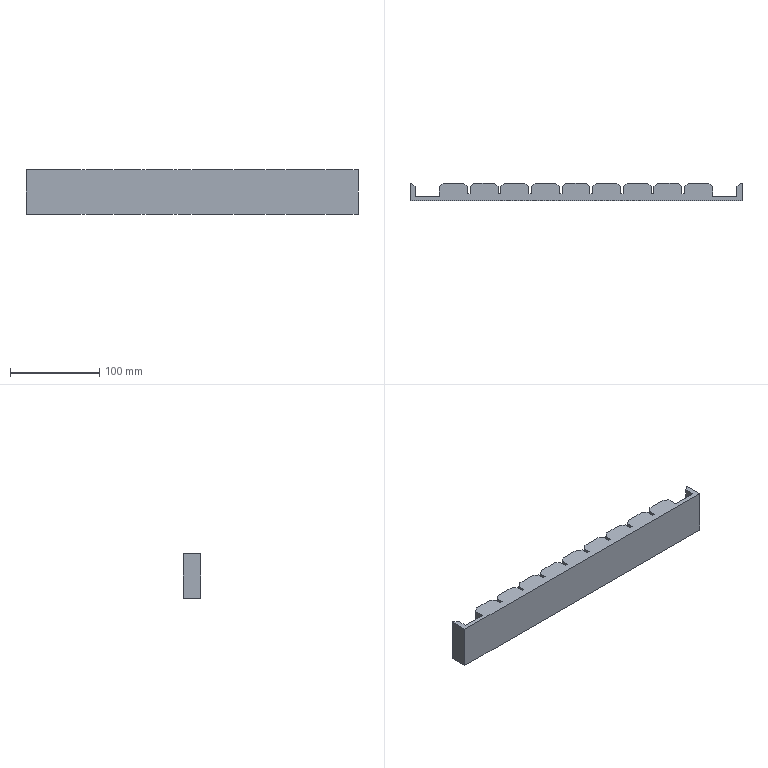NC program | NX | posted with a generic post | part box 372.9 x 20 x 50 mm
Lines 1 to 1463 of 3956:
N10 G17 G21 G94 G90
(FLOOR_WALL , TOOL : D6)
N12 T12 M6
N14 G54
N16 G17 G0 G90 X-164.156 Y-29.5 S9500 M3
N18 G43 Z30. H12
N20 Z0.904
N22 G94 G1 Z-0.596 F2500.
N24 X-166.58 Y-25.3
N26 G3 X-167.1 Y-25. R0.6
N28 G1 X-177.6
N30 Y25.
N32 X-156.6
N34 Y-25.
N36 X-167.1
N38 Y-22.
N40 X-174.6
N42 Y22.
N44 X-159.6
N46 Y-22.
N48 X-167.1
N50 Y-19.
N52 X-171.6
N54 Y19.
N56 X-162.6
N58 Y-19.
N60 X-167.1
N62 Y-16.
N64 X-168.6
N66 Y16.
N68 X-165.6
N70 Y-16.
N72 X-167.1
N74 G3 X-167.62 Y-16.3 R0.6
N76 G1 Z0.904
N78 G0 X-164.156 Y-29.5 Z0.308
N80 G1 Z-1.192
N82 X-166.58 Y-25.3
N84 G3 X-167.1 Y-25. R0.6
N86 G1 X-177.6
N88 Y25.
N90 X-156.6
N92 Y-25.
N94 X-167.1
N96 Y-22.
N98 X-174.6
N100 Y22.
N102 X-159.6
N104 Y-22.
N106 X-167.1
N108 Y-19.
N110 X-171.6
N112 Y19.
N114 X-162.6
N116 Y-19.
N118 X-167.1
N120 Y-16.
N122 X-168.6
N124 Y16.
N126 X-165.6
N128 Y-16.
N130 X-167.1
N132 G3 X-167.62 Y-16.3 R0.6
N134 G1 Z0.308
N136 G0 X-164.156 Y-29.5 Z-0.288
N138 G1 Z-1.788
N140 X-166.58 Y-25.3
N142 G3 X-167.1 Y-25. R0.6
N144 G1 X-177.6
N146 Y25.
N148 X-156.6
N150 Y-25.
N152 X-167.1
N154 Y-22.
N156 X-174.6
N158 Y22.
N160 X-159.6
N162 Y-22.
N164 X-167.1
N166 Y-19.
N168 X-171.6
N170 Y19.
N172 X-162.6
N174 Y-19.
N176 X-167.1
N178 Y-16.
N180 X-168.6
N182 Y16.
N184 X-165.6
N186 Y-16.
N188 X-167.1
N190 G3 X-167.62 Y-16.3 R0.6
N192 G1 Z-0.288
N194 G0 X-164.156 Y-29.5 Z-0.884
N196 G1 Z-2.384
N198 X-166.58 Y-25.3
N200 G3 X-167.1 Y-25. R0.6
N202 G1 X-177.6
N204 Y25.
N206 X-156.6
N208 Y-25.
N210 X-167.1
N212 Y-22.
N214 X-174.6
N216 Y22.
N218 X-159.6
N220 Y-22.
N222 X-167.1
N224 Y-19.
N226 X-171.6
N228 Y19.
N230 X-162.6
N232 Y-19.
N234 X-167.1
N236 Y-16.
N238 X-168.6
N240 Y16.
N242 X-165.6
N244 Y-16.
N246 X-167.1
N248 G3 X-167.62 Y-16.3 R0.6
N250 G1 Z-0.884
N252 G0 X-164.156 Y-29.5 Z-1.48
N254 G1 Z-2.98
N256 X-166.58 Y-25.3
N258 G3 X-167.1 Y-25. R0.6
N260 G1 X-177.6
N262 Y25.
N264 X-156.6
N266 Y-25.
N268 X-167.1
N270 Y-22.
N272 X-174.6
N274 Y22.
N276 X-159.6
N278 Y-22.
N280 X-167.1
N282 Y-19.
N284 X-171.6
N286 Y19.
N288 X-162.6
N290 Y-19.
N292 X-167.1
N294 Y-16.
N296 X-168.6
N298 Y16.
N300 X-165.6
N302 Y-16.
N304 X-167.1
N306 G3 X-167.62 Y-16.3 R0.6
N308 G1 Z-1.48
N310 G0 X-164.156 Y-29.5 Z-2.076
N312 G1 Z-3.576
N314 X-166.58 Y-25.3
N316 G3 X-167.1 Y-25. R0.6
N318 G1 X-177.6
N320 Y25.
N322 X-156.6
N324 Y-25.
N326 X-167.1
N328 Y-22.
N330 X-174.6
N332 Y22.
N334 X-159.6
N336 Y-22.
N338 X-167.1
N340 Y-19.
N342 X-171.6
N344 Y19.
N346 X-162.6
N348 Y-19.
N350 X-167.1
N352 Y-16.
N354 X-168.6
N356 Y16.
N358 X-165.6
N360 Y-16.
N362 X-167.1
N364 G3 X-167.62 Y-16.3 R0.6
N366 G1 Z-2.076
N368 G0 X-164.156 Y-29.5 Z-2.672
N370 G1 Z-4.172
N372 X-166.58 Y-25.3
N374 G3 X-167.1 Y-25. R0.6
N376 G1 X-177.6
N378 Y25.
N380 X-156.6
N382 Y-25.
N384 X-167.1
N386 Y-22.
N388 X-174.6
N390 Y22.
N392 X-159.6
N394 Y-22.
N396 X-167.1
N398 Y-19.
N400 X-171.6
N402 Y19.
N404 X-162.6
N406 Y-19.
N408 X-167.1
N410 Y-16.
N412 X-168.6
N414 Y16.
N416 X-165.6
N418 Y-16.
N420 X-167.1
N422 G3 X-167.62 Y-16.3 R0.6
N424 G1 Z-2.672
N426 G0 X-164.156 Y-29.5 Z-3.268
N428 G1 Z-4.768
N430 X-166.58 Y-25.3
N432 G3 X-167.1 Y-25. R0.6
N434 G1 X-177.6
N436 Y25.
N438 X-156.6
N440 Y-25.
N442 X-167.1
N444 Y-22.
N446 X-174.6
N448 Y22.
N450 X-159.6
N452 Y-22.
N454 X-167.1
N456 Y-19.
N458 X-171.6
N460 Y19.
N462 X-162.6
N464 Y-19.
N466 X-167.1
N468 Y-16.
N470 X-168.6
N472 Y16.
N474 X-165.6
N476 Y-16.
N478 X-167.1
N480 G3 X-167.62 Y-16.3 R0.6
N482 G1 Z-3.268
N484 G0 X-164.156 Y-29.5 Z-3.864
N486 G1 Z-5.364
N488 X-166.58 Y-25.3
N490 G3 X-167.1 Y-25. R0.6
N492 G1 X-177.6
N494 Y25.
N496 X-156.6
N498 Y-25.
N500 X-167.1
N502 Y-22.
N504 X-174.6
N506 Y22.
N508 X-159.6
N510 Y-22.
N512 X-167.1
N514 Y-19.
N516 X-171.6
N518 Y19.
N520 X-162.6
N522 Y-19.
N524 X-167.1
N526 Y-16.
N528 X-168.6
N530 Y16.
N532 X-165.6
N534 Y-16.
N536 X-167.1
N538 G3 X-167.62 Y-16.3 R0.6
N540 G1 Z-3.864
N542 G0 X-164.156 Y-29.5 Z-4.46
N544 G1 Z-5.96
N546 X-166.58 Y-25.3
N548 G3 X-167.1 Y-25. R0.6
N550 G1 X-177.6
N552 Y25.
N554 X-156.6
N556 Y-25.
N558 X-167.1
N560 Y-22.
N562 X-174.6
N564 Y22.
N566 X-159.6
N568 Y-22.
N570 X-167.1
N572 Y-19.
N574 X-171.6
N576 Y19.
N578 X-162.6
N580 Y-19.
N582 X-167.1
N584 Y-16.
N586 X-168.6
N588 Y16.
N590 X-165.6
N592 Y-16.
N594 X-167.1
N596 G3 X-167.62 Y-16.3 R0.6
N598 G1 Z-4.46
N600 G0 X-164.156 Y-29.5 Z-5.056
N602 G1 Z-6.556
N604 X-166.58 Y-25.3
N606 G3 X-167.1 Y-25. R0.6
N608 G1 X-177.6
N610 Y25.
N612 X-156.6
N614 Y-25.
N616 X-167.1
N618 Y-22.
N620 X-174.6
N622 Y22.
N624 X-159.6
N626 Y-22.
N628 X-167.1
N630 Y-19.
N632 X-171.6
N634 Y19.
N636 X-162.6
N638 Y-19.
N640 X-167.1
N642 Y-16.
N644 X-168.6
N646 Y16.
N648 X-165.6
N650 Y-16.
N652 X-167.1
N654 G3 X-167.62 Y-16.3 R0.6
N656 G1 Z-5.056
N658 G0 X-164.156 Y-29.5 Z-5.652
N660 G1 Z-7.152
N662 X-166.58 Y-25.3
N664 G3 X-167.1 Y-25. R0.6
N666 G1 X-177.6
N668 Y25.
N670 X-156.6
N672 Y-25.
N674 X-167.1
N676 Y-22.
N678 X-174.6
N680 Y22.
N682 X-159.6
N684 Y-22.
N686 X-167.1
N688 Y-19.
N690 X-171.6
N692 Y19.
N694 X-162.6
N696 Y-19.
N698 X-167.1
N700 Y-16.
N702 X-168.6
N704 Y16.
N706 X-165.6
N708 Y-16.
N710 X-167.1
N712 G3 X-167.62 Y-16.3 R0.6
N714 G1 Z-5.652
N716 G0 X-164.156 Y-29.5 Z-6.248
N718 G1 Z-7.748
N720 X-166.58 Y-25.3
N722 G3 X-167.1 Y-25. R0.6
N724 G1 X-177.6
N726 Y25.
N728 X-156.6
N730 Y-25.
N732 X-167.1
N734 Y-22.
N736 X-174.6
N738 Y22.
N740 X-159.6
N742 Y-22.
N744 X-167.1
N746 Y-19.
N748 X-171.6
N750 Y19.
N752 X-162.6
N754 Y-19.
N756 X-167.1
N758 Y-16.
N760 X-168.6
N762 Y16.
N764 X-165.6
N766 Y-16.
N768 X-167.1
N770 G3 X-167.62 Y-16.3 R0.6
N772 G1 Z-6.248
N774 G0 X-164.156 Y-29.5 Z-6.844
N776 G1 Z-8.344
N778 X-166.58 Y-25.3
N780 G3 X-167.1 Y-25. R0.6
N782 G1 X-177.6
N784 Y25.
N786 X-156.6
N788 Y-25.
N790 X-167.1
N792 Y-22.
N794 X-174.6
N796 Y22.
N798 X-159.6
N800 Y-22.
N802 X-167.1
N804 Y-19.
N806 X-171.6
N808 Y19.
N810 X-162.6
N812 Y-19.
N814 X-167.1
N816 Y-16.
N818 X-168.6
N820 Y16.
N822 X-165.6
N824 Y-16.
N826 X-167.1
N828 G3 X-167.62 Y-16.3 R0.6
N830 G1 Z-6.844
N832 G0 X-164.156 Y-29.5 Z-7.44
N834 G1 Z-8.94
N836 X-166.58 Y-25.3
N838 G3 X-167.1 Y-25. R0.6
N840 G1 X-177.6
N842 Y25.
N844 X-156.6
N846 Y-25.
N848 X-167.1
N850 Y-22.
N852 X-174.6
N854 Y22.
N856 X-159.6
N858 Y-22.
N860 X-167.1
N862 Y-19.
N864 X-171.6
N866 Y19.
N868 X-162.6
N870 Y-19.
N872 X-167.1
N874 Y-16.
N876 X-168.6
N878 Y16.
N880 X-165.6
N882 Y-16.
N884 X-167.1
N886 G3 X-167.62 Y-16.3 R0.6
N888 G1 Z-7.44
N890 G0 X-164.156 Y-29.5 Z-8.036
N892 G1 Z-9.536
N894 X-166.58 Y-25.3
N896 G3 X-167.1 Y-25. R0.6
N898 G1 X-177.6
N900 Y25.
N902 X-156.6
N904 Y-25.
N906 X-167.1
N908 Y-22.
N910 X-174.6
N912 Y22.
N914 X-159.6
N916 Y-22.
N918 X-167.1
N920 Y-19.
N922 X-171.6
N924 Y19.
N926 X-162.6
N928 Y-19.
N930 X-167.1
N932 Y-16.
N934 X-168.6
N936 Y16.
N938 X-165.6
N940 Y-16.
N942 X-167.1
N944 G3 X-167.62 Y-16.3 R0.6
N946 G1 Z-8.036
N948 G0 X-164.156 Y-29.5 Z-8.632
N950 G1 Z-10.132
N952 X-166.58 Y-25.3
N954 G3 X-167.1 Y-25. R0.6
N956 G1 X-177.6
N958 Y25.
N960 X-156.6
N962 Y-25.
N964 X-167.1
N966 Y-22.
N968 X-174.6
N970 Y22.
N972 X-159.6
N974 Y-22.
N976 X-167.1
N978 Y-19.
N980 X-171.6
N982 Y19.
N984 X-162.6
N986 Y-19.
N988 X-167.1
N990 Y-16.
N992 X-168.6
N994 Y16.
N996 X-165.6
N998 Y-16.
N1000 X-167.1
N1002 G3 X-167.62 Y-16.3 R0.6
N1004 G1 Z-8.632
N1006 G0 X-164.156 Y-29.5 Z-9.228
N1008 G1 Z-10.728
N1010 X-166.58 Y-25.3
N1012 G3 X-167.1 Y-25. R0.6
N1014 G1 X-177.6
N1016 Y25.
N1018 X-156.6
N1020 Y-25.
N1022 X-167.1
N1024 Y-22.
N1026 X-174.6
N1028 Y22.
N1030 X-159.6
N1032 Y-22.
N1034 X-167.1
N1036 Y-19.
N1038 X-171.6
N1040 Y19.
N1042 X-162.6
N1044 Y-19.
N1046 X-167.1
N1048 Y-16.
N1050 X-168.6
N1052 Y16.
N1054 X-165.6
N1056 Y-16.
N1058 X-167.1
N1060 G3 X-167.62 Y-16.3 R0.6
N1062 G1 Z-9.228
N1064 G0 X-164.156 Y-29.5 Z-9.824
N1066 G1 Z-11.324
N1068 X-166.58 Y-25.3
N1070 G3 X-167.1 Y-25. R0.6
N1072 G1 X-177.6
N1074 Y25.
N1076 X-156.6
N1078 Y-25.
N1080 X-167.1
N1082 Y-22.
N1084 X-174.6
N1086 Y22.
N1088 X-159.6
N1090 Y-22.
N1092 X-167.1
N1094 Y-19.
N1096 X-171.6
N1098 Y19.
N1100 X-162.6
N1102 Y-19.
N1104 X-167.1
N1106 Y-16.
N1108 X-168.6
N1110 Y16.
N1112 X-165.6
N1114 Y-16.
N1116 X-167.1
N1118 G3 X-167.62 Y-16.3 R0.6
N1120 G1 Z-9.824
N1122 G0 X-164.156 Y-29.5 Z-10.42
N1124 G1 Z-11.92
N1126 X-166.58 Y-25.3
N1128 G3 X-167.1 Y-25. R0.6
N1130 G1 X-177.6
N1132 Y25.
N1134 X-156.6
N1136 Y-25.
N1138 X-167.1
N1140 Y-22.
N1142 X-174.6
N1144 Y22.
N1146 X-159.6
N1148 Y-22.
N1150 X-167.1
N1152 Y-19.
N1154 X-171.6
N1156 Y19.
N1158 X-162.6
N1160 Y-19.
N1162 X-167.1
N1164 Y-16.
N1166 X-168.6
N1168 Y16.
N1170 X-165.6
N1172 Y-16.
N1174 X-167.1
N1176 G3 X-167.62 Y-16.3 R0.6
N1178 G1 Z-10.42
N1180 G0 X-164.156 Y-29.5 Z-11.016
N1182 G1 Z-12.516
N1184 X-166.58 Y-25.3
N1186 G3 X-167.1 Y-25. R0.6
N1188 G1 X-177.6
N1190 Y25.
N1192 X-156.6
N1194 Y-25.
N1196 X-167.1
N1198 Y-22.
N1200 X-174.6
N1202 Y22.
N1204 X-159.6
N1206 Y-22.
N1208 X-167.1
N1210 Y-19.
N1212 X-171.6
N1214 Y19.
N1216 X-162.6
N1218 Y-19.
N1220 X-167.1
N1222 Y-16.
N1224 X-168.6
N1226 Y16.
N1228 X-165.6
N1230 Y-16.
N1232 X-167.1
N1234 G3 X-167.62 Y-16.3 R0.6
N1236 G1 Z-11.016
N1238 G0 X-164.156 Y-29.5 Z-11.612
N1240 G1 Z-13.112
N1242 X-166.58 Y-25.3
N1244 G3 X-167.1 Y-25. R0.6
N1246 G1 X-177.6
N1248 Y25.
N1250 X-156.6
N1252 Y-25.
N1254 X-167.1
N1256 Y-22.
N1258 X-174.6
N1260 Y22.
N1262 X-159.6
N1264 Y-22.
N1266 X-167.1
N1268 Y-19.
N1270 X-171.6
N1272 Y19.
N1274 X-162.6
N1276 Y-19.
N1278 X-167.1
N1280 Y-16.
N1282 X-168.6
N1284 Y16.
N1286 X-165.6
N1288 Y-16.
N1290 X-167.1
N1292 G3 X-167.62 Y-16.3 R0.6
N1294 G1 Z-11.612
N1296 G0 X-164.156 Y-29.5 Z-12.208
N1298 G1 Z-13.708
N1300 X-166.58 Y-25.3
N1302 G3 X-167.1 Y-25. R0.6
N1304 G1 X-177.6
N1306 Y25.
N1308 X-156.6
N1310 Y-25.
N1312 X-167.1
N1314 Y-22.
N1316 X-174.6
N1318 Y22.
N1320 X-159.6
N1322 Y-22.
N1324 X-167.1
N1326 Y-19.
N1328 X-171.6
N1330 Y19.
N1332 X-162.6
N1334 Y-19.
N1336 X-167.1
N1338 Y-16.
N1340 X-168.6
N1342 Y16.
N1344 X-165.6
N1346 Y-16.
N1348 X-167.1
N1350 G3 X-167.62 Y-16.3 R0.6
N1352 G1 Z-12.208
N1354 G0 X-164.156 Y-29.5 Z-12.804
N1356 G1 Z-14.304
N1358 X-166.58 Y-25.3
N1360 G3 X-167.1 Y-25. R0.6
N1362 G1 X-177.6
N1364 Y25.
N1366 X-156.6
N1368 Y-25.
N1370 X-167.1
N1372 Y-22.
N1374 X-174.6
N1376 Y22.
N1378 X-159.6
N1380 Y-22.
N1382 X-167.1
N1384 Y-19.
N1386 X-171.6
N1388 Y19.
N1390 X-162.6
N1392 Y-19.
N1394 X-167.1
N1396 Y-16.
N1398 X-168.6
N1400 Y16.
N1402 X-165.6
N1404 Y-16.
N1406 X-167.1
N1408 G3 X-167.62 Y-16.3 R0.6
N1410 G1 Z-12.804
N1412 G0 X-164.156 Y-29.5 Z-13.4
N1414 G1 Z-14.9
N1416 X-166.58 Y-25.3
N1418 G3 X-167.1 Y-25. R0.6
N1420 G1 X-177.6
N1422 Y25.
N1424 X-156.6
N1426 Y-25.
N1428 X-167.1
N1430 Y-22.
N1432 X-174.6
N1434 Y22.
N1436 X-159.6
N1438 Y-22.
N1440 X-167.1
N1442 Y-19.
N1444 X-171.6
N1446 Y19.
N1448 X-162.6
N1450 Y-19.
N1452 X-167.1
N1454 Y-16.
N1456 X-168.6
N1458 Y16.
N1460 X-165.6
N1462 Y-16.
N1464 X-167.1
N1466 G3 X-167.62 Y-16.3 R0.6
N1468 G1 Z-13.4
N1470 G0 Z30.
N1472 X170.044 Y-29.5
N1474 Z0.904
N1476 G1 Z-0.596
N1478 X167.62 Y-25.3
N1480 G3 X167.1 Y-25. R0.6
N1482 G1 X156.6
N1484 Y25.
N1486 X177.6
N1488 Y-25.
N1490 X167.1
N1492 Y-22.
N1494 X159.6
N1496 Y22.
N1498 X174.6
N1500 Y-22.
N1502 X167.1
N1504 Y-19.
N1506 X162.6
N1508 Y19.
N1510 X171.6
N1512 Y-19.
N1514 X167.1
N1516 Y-16.
N1518 X165.6
N1520 Y16.
N1522 X168.6
N1524 Y-16.
N1526 X167.1
N1528 G3 X166.58 Y-16.3 R0.6
N1530 G1 Z0.904
N1532 G0 X170.044 Y-29.5 Z0.308
N1534 G1 Z-1.192
N1536 X167.62 Y-25.3
N1538 G3 X167.1 Y-25. R0.6
N1540 G1 X156.6
N1542 Y25.
N1544 X177.6
N1546 Y-25.
N1548 X167.1
N1550 Y-22.
N1552 X159.6
N1554 Y22.
N1556 X174.6
N1558 Y-22.
N1560 X167.1
N1562 Y-19.
N1564 X162.6
N1566 Y19.
N1568 X171.6
N1570 Y-19.
N1572 X167.1
N1574 Y-16.
N1576 X165.6
N1578 Y16.
N1580 X168.6
N1582 Y-16.
N1584 X167.1
N1586 G3 X166.58 Y-16.3 R0.6
N1588 G1 Z0.308
N1590 G0 X170.044 Y-29.5 Z-0.288
N1592 G1 Z-1.788
N1594 X167.62 Y-25.3
N1596 G3 X167.1 Y-25. R0.6
N1598 G1 X156.6
N1600 Y25.
N1602 X177.6
N1604 Y-25.
N1606 X167.1
N1608 Y-22.
N1610 X159.6
N1612 Y22.
N1614 X174.6
N1616 Y-22.
N1618 X167.1
N1620 Y-19.
N1622 X162.6
N1624 Y19.
N1626 X171.6
N1628 Y-19.
N1630 X167.1
N1632 Y-16.
N1634 X165.6
N1636 Y16.
N1638 X168.6
N1640 Y-16.
N1642 X167.1
N1644 G3 X166.58 Y-16.3 R0.6
N1646 G1 Z-0.288
N1648 G0 X170.044 Y-29.5 Z-0.884
N1650 G1 Z-2.384
N1652 X167.62 Y-25.3
N1654 G3 X167.1 Y-25. R0.6
N1656 G1 X156.6
N1658 Y25.
N1660 X177.6
N1662 Y-25.
N1664 X167.1
N1666 Y-22.
N1668 X159.6
N1670 Y22.
N1672 X174.6
N1674 Y-22.
N1676 X167.1
N1678 Y-19.
N1680 X162.6
N1682 Y19.
N1684 X171.6
N1686 Y-19.
N1688 X167.1
N1690 Y-16.
N1692 X165.6
N1694 Y16.
N1696 X168.6
N1698 Y-16.
N1700 X167.1
N1702 G3 X166.58 Y-16.3 R0.6
N1704 G1 Z-0.884
N1706 G0 X170.044 Y-29.5 Z-1.48
N1708 G1 Z-2.98
N1710 X167.62 Y-25.3
N1712 G3 X167.1 Y-25. R0.6
N1714 G1 X156.6
N1716 Y25.
N1718 X177.6
N1720 Y-25.
N1722 X167.1
N1724 Y-22.
N1726 X159.6
N1728 Y22.
N1730 X174.6
N1732 Y-22.
N1734 X167.1
N1736 Y-19.
N1738 X162.6
N1740 Y19.
N1742 X171.6
N1744 Y-19.
N1746 X167.1
N1748 Y-16.
N1750 X165.6
N1752 Y16.
N1754 X168.6
N1756 Y-16.
N1758 X167.1
N1760 G3 X166.58 Y-16.3 R0.6
N1762 G1 Z-1.48
N1764 G0 X170.044 Y-29.5 Z-2.076
N1766 G1 Z-3.576
N1768 X167.62 Y-25.3
N1770 G3 X167.1 Y-25. R0.6
N1772 G1 X156.6
N1774 Y25.
N1776 X177.6
N1778 Y-25.
N1780 X167.1
N1782 Y-22.
N1784 X159.6
N1786 Y22.
N1788 X174.6
N1790 Y-22.
N1792 X167.1
N1794 Y-19.
N1796 X162.6
N1798 Y19.
N1800 X171.6
N1802 Y-19.
N1804 X167.1
N1806 Y-16.
N1808 X165.6
N1810 Y16.
N1812 X168.6
N1814 Y-16.
N1816 X167.1
N1818 G3 X166.58 Y-16.3 R0.6
N1820 G1 Z-2.076
N1822 G0 X170.044 Y-29.5 Z-2.672
N1824 G1 Z-4.172
N1826 X167.62 Y-25.3
N1828 G3 X167.1 Y-25. R0.6
N1830 G1 X156.6
N1832 Y25.
N1834 X177.6
N1836 Y-25.
N1838 X167.1
N1840 Y-22.
N1842 X159.6
N1844 Y22.
N1846 X174.6
N1848 Y-22.
N1850 X167.1
N1852 Y-19.
N1854 X162.6
N1856 Y19.
N1858 X171.6
N1860 Y-19.
N1862 X167.1
N1864 Y-16.
N1866 X165.6
N1868 Y16.
N1870 X168.6
N1872 Y-16.
N1874 X167.1
N1876 G3 X166.58 Y-16.3 R0.6
N1878 G1 Z-2.672
N1880 G0 X170.044 Y-29.5 Z-3.268
N1882 G1 Z-4.768
N1884 X167.62 Y-25.3
N1886 G3 X167.1 Y-25. R0.6
N1888 G1 X156.6
N1890 Y25.
N1892 X177.6
N1894 Y-25.
N1896 X167.1
N1898 Y-22.
N1900 X159.6
N1902 Y22.
N1904 X174.6
N1906 Y-22.
N1908 X167.1
N1910 Y-19.
N1912 X162.6
N1914 Y19.
N1916 X171.6
N1918 Y-19.
N1920 X167.1
N1922 Y-16.
N1924 X165.6
N1926 Y16.
N1928 X168.6
N1930 Y-16.
N1932 X167.1
N1934 G3 X166.58 Y-16.3 R0.6
N1936 G1 Z-3.268
N1938 G0 X170.044 Y-29.5 Z-3.864
N1940 G1 Z-5.364
N1942 X167.62 Y-25.3
N1944 G3 X167.1 Y-25. R0.6
N1946 G1 X156.6
N1948 Y25.
N1950 X177.6
N1952 Y-25.
N1954 X167.1
N1956 Y-22.
N1958 X159.6
N1960 Y22.
N1962 X174.6
N1964 Y-22.
N1966 X167.1
N1968 Y-19.
N1970 X162.6
N1972 Y19.
N1974 X171.6
N1976 Y-19.
N1978 X167.1
N1980 Y-16.
N1982 X165.6
N1984 Y16.
N1986 X168.6
N1988 Y-16.
N1990 X167.1
N1992 G3 X166.58 Y-16.3 R0.6
N1994 G1 Z-3.864
N1996 G0 X170.044 Y-29.5 Z-4.46
N1998 G1 Z-5.96
N2000 X167.62 Y-25.3
N2002 G3 X167.1 Y-25. R0.6
N2004 G1 X156.6
N2006 Y25.
N2008 X177.6
N2010 Y-25.
N2012 X167.1
N2014 Y-22.
N2016 X159.6
N2018 Y22.
N2020 X174.6
N2022 Y-22.
N2024 X167.1
N2026 Y-19.
N2028 X162.6
N2030 Y19.
N2032 X171.6
N2034 Y-19.
N2036 X167.1
N2038 Y-16.
N2040 X165.6
N2042 Y16.
N2044 X168.6
N2046 Y-16.
N2048 X167.1
N2050 G3 X166.58 Y-16.3 R0.6
N2052 G1 Z-4.46
N2054 G0 X170.044 Y-29.5 Z-5.056
N2056 G1 Z-6.556
N2058 X167.62 Y-25.3
N2060 G3 X167.1 Y-25. R0.6
N2062 G1 X156.6
N2064 Y25.
N2066 X177.6
N2068 Y-25.
N2070 X167.1
N2072 Y-22.
N2074 X159.6
N2076 Y22.
N2078 X174.6
N2080 Y-22.
N2082 X167.1
N2084 Y-19.
N2086 X162.6
N2088 Y19.
N2090 X171.6
N2092 Y-19.
N2094 X167.1
N2096 Y-16.
N2098 X165.6
N2100 Y16.
N2102 X168.6
N2104 Y-16.
N2106 X167.1
N2108 G3 X166.58 Y-16.3 R0.6
N2110 G1 Z-5.056
N2112 G0 X170.044 Y-29.5 Z-5.652
N2114 G1 Z-7.152
N2116 X167.62 Y-25.3
N2118 G3 X167.1 Y-25. R0.6
N2120 G1 X156.6
N2122 Y25.
N2124 X177.6
N2126 Y-25.
N2128 X167.1
N2130 Y-22.
N2132 X159.6
N2134 Y22.
N2136 X174.6
N2138 Y-22.
N2140 X167.1
N2142 Y-19.
N2144 X162.6
N2146 Y19.
N2148 X171.6
N2150 Y-19.
N2152 X167.1
N2154 Y-16.
N2156 X165.6
N2158 Y16.
N2160 X168.6
N2162 Y-16.
N2164 X167.1
N2166 G3 X166.58 Y-16.3 R0.6
N2168 G1 Z-5.652
N2170 G0 X170.044 Y-29.5 Z-6.248
N2172 G1 Z-7.748
N2174 X167.62 Y-25.3
N2176 G3 X167.1 Y-25. R0.6
N2178 G1 X156.6
N2180 Y25.
N2182 X177.6
N2184 Y-25.
N2186 X167.1
N2188 Y-22.
N2190 X159.6
N2192 Y22.
N2194 X174.6
N2196 Y-22.
N2198 X167.1
N2200 Y-19.
N2202 X162.6
N2204 Y19.
N2206 X171.6
N2208 Y-19.
N2210 X167.1
N2212 Y-16.
N2214 X165.6
N2216 Y16.
N2218 X168.6
N2220 Y-16.
N2222 X167.1
N2224 G3 X166.58 Y-16.3 R0.6
N2226 G1 Z-6.248
N2228 G0 X170.044 Y-29.5 Z-6.844
N2230 G1 Z-8.344
N2232 X167.62 Y-25.3
N2234 G3 X167.1 Y-25. R0.6
N2236 G1 X156.6
N2238 Y25.
N2240 X177.6
N2242 Y-25.
N2244 X167.1
N2246 Y-22.
N2248 X159.6
N2250 Y22.
N2252 X174.6
N2254 Y-22.
N2256 X167.1
N2258 Y-19.
N2260 X162.6
N2262 Y19.
N2264 X171.6
N2266 Y-19.
N2268 X167.1
N2270 Y-16.
N2272 X165.6
N2274 Y16.
N2276 X168.6
N2278 Y-16.
N2280 X167.1
N2282 G3 X166.58 Y-16.3 R0.6
N2284 G1 Z-6.844
N2286 G0 X170.044 Y-29.5 Z-7.44
N2288 G1 Z-8.94
N2290 X167.62 Y-25.3
N2292 G3 X167.1 Y-25. R0.6
N2294 G1 X156.6
N2296 Y25.
N2298 X177.6
N2300 Y-25.
N2302 X167.1
N2304 Y-22.
N2306 X159.6
N2308 Y22.
N2310 X174.6
N2312 Y-22.
N2314 X167.1
N2316 Y-19.
N2318 X162.6
N2320 Y19.
N2322 X171.6
N2324 Y-19.
N2326 X167.1
N2328 Y-16.
N2330 X165.6
N2332 Y16.
N2334 X168.6
N2336 Y-16.
N2338 X167.1
N2340 G3 X166.58 Y-16.3 R0.6
N2342 G1 Z-7.44
N2344 G0 X170.044 Y-29.5 Z-8.036
N2346 G1 Z-9.536
N2348 X167.62 Y-25.3
N2350 G3 X167.1 Y-25. R0.6
N2352 G1 X156.6
N2354 Y25.
N2356 X177.6
N2358 Y-25.
N2360 X167.1
N2362 Y-22.
N2364 X159.6
N2366 Y22.
N2368 X174.6
N2370 Y-22.
N2372 X167.1
N2374 Y-19.
N2376 X162.6
N2378 Y19.
N2380 X171.6
N2382 Y-19.
N2384 X167.1
N2386 Y-16.
N2388 X165.6
N2390 Y16.
N2392 X168.6
N2394 Y-16.
N2396 X167.1
N2398 G3 X166.58 Y-16.3 R0.6
N2400 G1 Z-8.036
N2402 G0 X170.044 Y-29.5 Z-8.632
N2404 G1 Z-10.132
N2406 X167.62 Y-25.3
N2408 G3 X167.1 Y-25. R0.6
N2410 G1 X156.6
N2412 Y25.
N2414 X177.6
N2416 Y-25.
N2418 X167.1
N2420 Y-22.
N2422 X159.6
N2424 Y22.
N2426 X174.6
N2428 Y-22.
N2430 X167.1
N2432 Y-19.
N2434 X162.6
N2436 Y19.
N2438 X171.6
N2440 Y-19.
N2442 X167.1
N2444 Y-16.
N2446 X165.6
N2448 Y16.
N2450 X168.6
N2452 Y-16.
N2454 X167.1
N2456 G3 X166.58 Y-16.3 R0.6
N2458 G1 Z-8.632
N2460 G0 X170.044 Y-29.5 Z-9.228
N2462 G1 Z-10.728
N2464 X167.62 Y-25.3
N2466 G3 X167.1 Y-25. R0.6
N2468 G1 X156.6
N2470 Y25.
N2472 X177.6
N2474 Y-25.
N2476 X167.1
N2478 Y-22.
N2480 X159.6
N2482 Y22.
N2484 X174.6
N2486 Y-22.
N2488 X167.1
N2490 Y-19.
N2492 X162.6
N2494 Y19.
N2496 X171.6
N2498 Y-19.
N2500 X167.1
N2502 Y-16.
N2504 X165.6
N2506 Y16.
N2508 X168.6
N2510 Y-16.
N2512 X167.1
N2514 G3 X166.58 Y-16.3 R0.6
N2516 G1 Z-9.228
N2518 G0 X170.044 Y-29.5 Z-9.824
N2520 G1 Z-11.324
N2522 X167.62 Y-25.3
N2524 G3 X167.1 Y-25. R0.6
N2526 G1 X156.6
N2528 Y25.
N2530 X177.6
N2532 Y-25.
N2534 X167.1
N2536 Y-22.
N2538 X159.6
N2540 Y22.
N2542 X174.6
N2544 Y-22.
N2546 X167.1
N2548 Y-19.
N2550 X162.6
N2552 Y19.
N2554 X171.6
N2556 Y-19.
N2558 X167.1
N2560 Y-16.
N2562 X165.6
N2564 Y16.
N2566 X168.6
N2568 Y-16.
N2570 X167.1
N2572 G3 X166.58 Y-16.3 R0.6
N2574 G1 Z-9.824
N2576 G0 X170.044 Y-29.5 Z-10.42
N2578 G1 Z-11.92
N2580 X167.62 Y-25.3
N2582 G3 X167.1 Y-25. R0.6
N2584 G1 X156.6
N2586 Y25.
N2588 X177.6
N2590 Y-25.
N2592 X167.1
N2594 Y-22.
N2596 X159.6
N2598 Y22.
N2600 X174.6
N2602 Y-22.
N2604 X167.1
N2606 Y-19.
N2608 X162.6
N2610 Y19.
N2612 X171.6
N2614 Y-19.
N2616 X167.1
N2618 Y-16.
N2620 X165.6
N2622 Y16.
N2624 X168.6
N2626 Y-16.
N2628 X167.1
N2630 G3 X166.58 Y-16.3 R0.6
N2632 G1 Z-10.42
N2634 G0 X170.044 Y-29.5 Z-11.016
N2636 G1 Z-12.516
N2638 X167.62 Y-25.3
N2640 G3 X167.1 Y-25. R0.6
N2642 G1 X156.6
N2644 Y25.
N2646 X177.6
N2648 Y-25.
N2650 X167.1
N2652 Y-22.
N2654 X159.6
N2656 Y22.
N2658 X174.6
N2660 Y-22.
N2662 X167.1
N2664 Y-19.
N2666 X162.6
N2668 Y19.
N2670 X171.6
N2672 Y-19.
N2674 X167.1
N2676 Y-16.
N2678 X165.6
N2680 Y16.
N2682 X168.6
N2684 Y-16.
N2686 X167.1
N2688 G3 X166.58 Y-16.3 R0.6
N2690 G1 Z-11.016
N2692 G0 X170.044 Y-29.5 Z-11.612
N2694 G1 Z-13.112
N2696 X167.62 Y-25.3
N2698 G3 X167.1 Y-25. R0.6
N2700 G1 X156.6
N2702 Y25.
N2704 X177.6
N2706 Y-25.
N2708 X167.1
N2710 Y-22.
N2712 X159.6
N2714 Y22.
N2716 X174.6
N2718 Y-22.
N2720 X167.1
N2722 Y-19.
N2724 X162.6
N2726 Y19.
N2728 X171.6
N2730 Y-19.
N2732 X167.1
N2734 Y-16.
N2736 X165.6
N2738 Y16.
N2740 X168.6
N2742 Y-16.
N2744 X167.1
N2746 G3 X166.58 Y-16.3 R0.6
N2748 G1 Z-11.612
N2750 G0 X170.044 Y-29.5 Z-12.208
N2752 G1 Z-13.708
N2754 X167.62 Y-25.3
N2756 G3 X167.1 Y-25. R0.6
N2758 G1 X156.6
N2760 Y25.
N2762 X177.6
N2764 Y-25.
N2766 X167.1
N2768 Y-22.
N2770 X159.6
N2772 Y22.
N2774 X174.6
N2776 Y-22.
N2778 X167.1
N2780 Y-19.
N2782 X162.6
N2784 Y19.
N2786 X171.6
N2788 Y-19.
N2790 X167.1
N2792 Y-16.
N2794 X165.6
N2796 Y16.
N2798 X168.6
N2800 Y-16.
N2802 X167.1
N2804 G3 X166.58 Y-16.3 R0.6
N2806 G1 Z-12.208
N2808 G0 X170.044 Y-29.5 Z-12.804
N2810 G1 Z-14.304
N2812 X167.62 Y-25.3
N2814 G3 X167.1 Y-25. R0.6
N2816 G1 X156.6
N2818 Y25.
N2820 X177.6
N2822 Y-25.
N2824 X167.1
N2826 Y-22.
N2828 X159.6
N2830 Y22.
N2832 X174.6
N2834 Y-22.
N2836 X167.1
N2838 Y-19.
N2840 X162.6
N2842 Y19.
N2844 X171.6
N2846 Y-19.
N2848 X167.1
N2850 Y-16.
N2852 X165.6
N2854 Y16.
N2856 X168.6
N2858 Y-16.
N2860 X167.1
N2862 G3 X166.58 Y-16.3 R0.6
N2864 G1 Z-12.804
N2866 G0 X170.044 Y-29.5 Z-13.4
N2868 G1 Z-14.9
N2870 X167.62 Y-25.3
N2872 G3 X167.1 Y-25. R0.6
N2874 G1 X156.6
N2876 Y25.
N2878 X177.6
N2880 Y-25.
N2882 X167.1
N2884 Y-22.
N2886 X159.6
N2888 Y22.
N2890 X174.6
N2892 Y-22.
N2894 X167.1
N2896 Y-19.
N2898 X162.6
N2900 Y19.
N2902 X171.6
N2904 Y-19.
N2906 X167.1
N2908 Y-16.
N2910 X165.6
N2912 Y16.
N2914 X168.6
N2916 Y-16.
N2918 X167.1
N2920 G3 X166.58 Y-16.3 R0.6
N2922 G1 Z-13.4
N2924 G0 Z30.